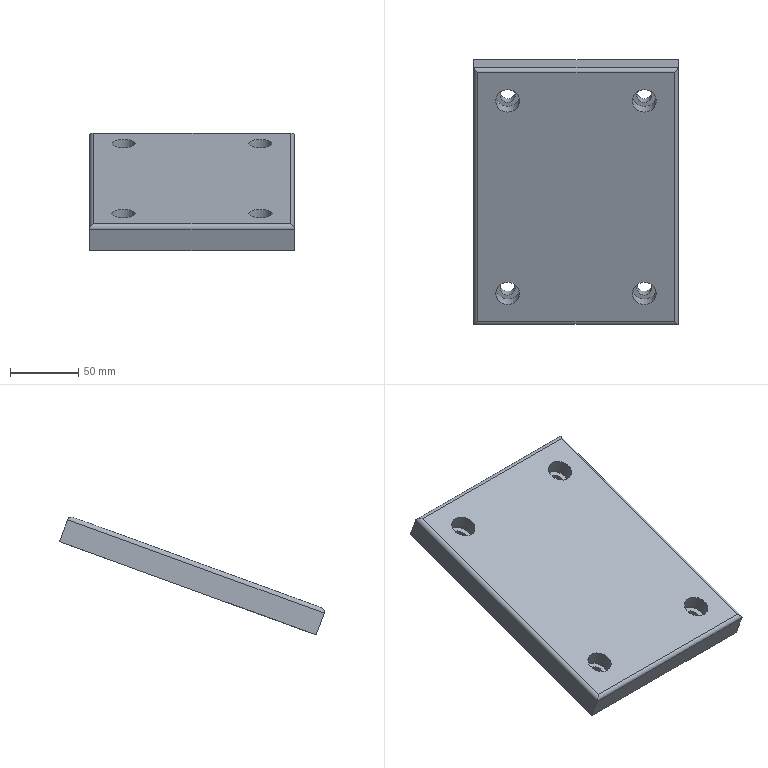Part | NX | features solid 2 | 1 solid | 22 faces | box 150 x 193.934 x 86.353 mm | volume 584072 mm3 | cylinder 12 | plane 10 | commonest cylinder face diameters 6 x4 11 x4 17.5 x4
STEP:
#1=CARTESIAN_POINT('',(72.,812.613,-309.301));
#2=VERTEX_POINT('',#1);
#3=CARTESIAN_POINT('',(-72.,812.613,-309.301));
#4=VERTEX_POINT('',#3);
#5=CARTESIAN_POINT('',(-37.6,812.613,-309.301));
#6=DIRECTION('',(-1.,0.,0.));
#7=VECTOR('',#6,1000.);
#8=LINE('',#5,#7);
#9=EDGE_CURVE('',#2,#4,#8,.T.);
#10=ORIENTED_EDGE('',*,*,#9,.T.);
#11=CARTESIAN_POINT('',(-75.,810.82,-313.146));
#12=VERTEX_POINT('',#11);
#13=CARTESIAN_POINT('',(-72.,813.639,-312.12));
#14=DIRECTION('',(0.7071,-0.6645,-0.2418));
#15=DIRECTION('',(-0.7071,-0.6645,-0.2418));
#16=AXIS2_PLACEMENT_3D('',#13,#14,#15);
#17=ELLIPSE('',#16,4.243,3.);
#18=EDGE_CURVE('',#4,#12,#17,.T.);
#19=ORIENTED_EDGE('',*,*,#18,.T.);
#20=CARTESIAN_POINT('',(75.,810.82,-313.146));
#21=VERTEX_POINT('',#20);
#22=CARTESIAN_POINT('',(78.95,810.82,-313.146));
#23=DIRECTION('',(-1.,0.,0.));
#24=VECTOR('',#23,1000.);
#25=LINE('',#22,#24);
#26=EDGE_CURVE('',#12,#21,#25,.F.);
#27=ORIENTED_EDGE('',*,*,#26,.T.);
#28=CARTESIAN_POINT('',(72.,813.639,-312.12));
#29=DIRECTION('',(0.7071,0.6645,0.2418));
#30=DIRECTION('',(0.7071,-0.6645,-0.2418));
#31=AXIS2_PLACEMENT_3D('',#28,#29,#30);
#32=ELLIPSE('',#31,4.243,3.);
#33=EDGE_CURVE('',#2,#21,#32,.T.);
#34=ORIENTED_EDGE('',*,*,#33,.F.);
#35=EDGE_LOOP('',(#10,#19,#27,#34));
#36=FACE_BOUND('',#35,.T.);
#37=CARTESIAN_POINT('',(-37.6,813.639,-312.12));
#38=DIRECTION('',(-1.,0.,0.));
#39=DIRECTION('',(0.,1.,0.));
#40=AXIS2_PLACEMENT_3D('',#37,#38,#39);
#41=CYLINDRICAL_SURFACE('',#40,3.);
#42=ADVANCED_FACE('',(#36),#41,.T.);
#43=CARTESIAN_POINT('',(-50.,966.018,-253.466));
#44=VERTEX_POINT('',#43);
#45=CARTESIAN_POINT('',(-50.,974.24,-250.474));
#46=DIRECTION('',(0.,0.342,-0.9397));
#47=DIRECTION('',(0.,-0.9397,-0.342));
#48=AXIS2_PLACEMENT_3D('',#45,#46,#47);
#49=CIRCLE('',#48,8.75);
#50=EDGE_CURVE('',#44,#44,#49,.F.);
#51=ORIENTED_EDGE('',*,*,#50,.F.);
#52=EDGE_LOOP('',(#51));
#53=FACE_BOUND('',#52,.T.);
#54=CARTESIAN_POINT('',(-50.,841.508,-298.784));
#55=VERTEX_POINT('',#54);
#56=CARTESIAN_POINT('',(-50.,833.286,-301.777));
#57=DIRECTION('',(0.,-0.342,0.9397));
#58=DIRECTION('',(0.,0.9397,0.342));
#59=AXIS2_PLACEMENT_3D('',#56,#57,#58);
#60=CIRCLE('',#59,8.75);
#61=EDGE_CURVE('',#55,#55,#60,.T.);
#62=ORIENTED_EDGE('',*,*,#61,.F.);
#63=EDGE_LOOP('',(#62));
#64=FACE_BOUND('',#63,.T.);
#65=CARTESIAN_POINT('',(-72.,994.913,-242.949));
#66=VERTEX_POINT('',#65);
#67=CARTESIAN_POINT('',(72.,994.913,-242.949));
#68=VERTEX_POINT('',#67);
#69=CARTESIAN_POINT('',(-37.6,994.913,-242.949));
#70=DIRECTION('',(-1.,0.,0.));
#71=VECTOR('',#70,1000.);
#72=LINE('',#69,#71);
#73=EDGE_CURVE('',#66,#68,#72,.F.);
#74=ORIENTED_EDGE('',*,*,#73,.F.);
#75=CARTESIAN_POINT('',(-72.,809.606,-310.396));
#76=DIRECTION('',(0.,0.9397,0.342));
#77=VECTOR('',#76,1000.);
#78=LINE('',#75,#77);
#79=EDGE_CURVE('',#4,#66,#78,.T.);
#80=ORIENTED_EDGE('',*,*,#79,.F.);
#81=ORIENTED_EDGE('',*,*,#9,.F.);
#82=CARTESIAN_POINT('',(72.,809.606,-310.396));
#83=DIRECTION('',(0.,0.9397,0.342));
#84=VECTOR('',#83,1000.);
#85=LINE('',#82,#84);
#86=EDGE_CURVE('',#2,#68,#85,.T.);
#87=ORIENTED_EDGE('',*,*,#86,.T.);
#88=EDGE_LOOP('',(#74,#80,#81,#87));
#89=FACE_BOUND('',#88,.T.);
#90=CARTESIAN_POINT('',(50.,966.018,-253.466));
#91=VERTEX_POINT('',#90);
#92=CARTESIAN_POINT('',(50.,974.24,-250.474));
#93=DIRECTION('',(0.,-0.342,0.9397));
#94=DIRECTION('',(0.,-0.9397,-0.342));
#95=AXIS2_PLACEMENT_3D('',#92,#93,#94);
#96=CIRCLE('',#95,8.75);
#97=EDGE_CURVE('',#91,#91,#96,.F.);
#98=ORIENTED_EDGE('',*,*,#97,.T.);
#99=EDGE_LOOP('',(#98));
#100=FACE_BOUND('',#99,.T.);
#101=CARTESIAN_POINT('',(50.,841.508,-298.784));
#102=VERTEX_POINT('',#101);
#103=CARTESIAN_POINT('',(50.,833.286,-301.777));
#104=DIRECTION('',(0.,0.342,-0.9397));
#105=DIRECTION('',(0.,0.9397,0.342));
#106=AXIS2_PLACEMENT_3D('',#103,#104,#105);
#107=CIRCLE('',#106,8.75);
#108=EDGE_CURVE('',#102,#102,#107,.T.);
#109=ORIENTED_EDGE('',*,*,#108,.T.);
#110=EDGE_LOOP('',(#109));
#111=FACE_BOUND('',#110,.T.);
#112=CARTESIAN_POINT('',(-37.6,809.606,-310.396));
#113=DIRECTION('',(0.,-0.342,0.9397));
#114=DIRECTION('',(0.,0.9397,0.342));
#115=AXIS2_PLACEMENT_3D('',#112,#113,#114);
#116=PLANE('',#115);
#117=ADVANCED_FACE('',(#53,#64,#89,#100,#111),#116,.T.);
#118=ORIENTED_EDGE('',*,*,#26,.F.);
#119=CARTESIAN_POINT('',(-75.,816.634,-329.121));
#120=VERTEX_POINT('',#119);
#121=CARTESIAN_POINT('',(-75.,817.01,-330.155));
#122=DIRECTION('',(0.,-0.342,0.9397));
#123=VECTOR('',#122,1000.);
#124=LINE('',#121,#123);
#125=EDGE_CURVE('',#120,#12,#124,.T.);
#126=ORIENTED_EDGE('',*,*,#125,.F.);
#127=CARTESIAN_POINT('',(75.,816.634,-329.121));
#128=VERTEX_POINT('',#127);
#129=CARTESIAN_POINT('',(-37.5,816.634,-329.121));
#130=DIRECTION('',(1.,0.,0.));
#131=VECTOR('',#130,1000.);
#132=LINE('',#129,#131);
#133=EDGE_CURVE('',#120,#128,#132,.T.);
#134=ORIENTED_EDGE('',*,*,#133,.T.);
#135=CARTESIAN_POINT('',(75.,817.01,-330.155));
#136=DIRECTION('',(0.,-0.342,0.9397));
#137=VECTOR('',#136,1000.);
#138=LINE('',#135,#137);
#139=EDGE_CURVE('',#128,#21,#138,.T.);
#140=ORIENTED_EDGE('',*,*,#139,.T.);
#141=EDGE_LOOP('',(#118,#126,#134,#140));
#142=FACE_BOUND('',#141,.T.);
#143=CARTESIAN_POINT('',(78.95,817.01,-330.155));
#144=DIRECTION('',(0.,-0.9397,-0.342));
#145=DIRECTION('',(-1.,0.,0.));
#146=AXIS2_PLACEMENT_3D('',#143,#144,#145);
#147=PLANE('',#146);
#148=ADVANCED_FACE('',(#142),#147,.T.);
#149=CARTESIAN_POINT('',(-50.,986.249,-267.387));
#150=VERTEX_POINT('',#149);
#151=CARTESIAN_POINT('',(-50.,981.08,-269.268));
#152=DIRECTION('',(0.,-0.342,0.9397));
#153=DIRECTION('',(0.,0.9397,0.342));
#154=AXIS2_PLACEMENT_3D('',#151,#152,#153);
#155=CIRCLE('',#154,5.5);
#156=EDGE_CURVE('',#150,#150,#155,.T.);
#157=ORIENTED_EDGE('',*,*,#156,.T.);
#158=EDGE_LOOP('',(#157));
#159=FACE_BOUND('',#158,.T.);
#160=CARTESIAN_POINT('',(-50.,845.295,-318.69));
#161=VERTEX_POINT('',#160);
#162=CARTESIAN_POINT('',(-50.,840.126,-320.571));
#163=DIRECTION('',(0.,-0.342,0.9397));
#164=DIRECTION('',(0.,0.9397,0.342));
#165=AXIS2_PLACEMENT_3D('',#162,#163,#164);
#166=CIRCLE('',#165,5.5);
#167=EDGE_CURVE('',#161,#161,#166,.T.);
#168=ORIENTED_EDGE('',*,*,#167,.T.);
#169=EDGE_LOOP('',(#168));
#170=FACE_BOUND('',#169,.T.);
#171=ORIENTED_EDGE('',*,*,#133,.F.);
#172=CARTESIAN_POINT('',(-75.,1004.573,-260.717));
#173=VERTEX_POINT('',#172);
#174=CARTESIAN_POINT('',(-75.,816.446,-329.19));
#175=DIRECTION('',(0.,-0.9397,-0.342));
#176=VECTOR('',#175,1000.);
#177=LINE('',#174,#176);
#178=EDGE_CURVE('',#173,#120,#177,.T.);
#179=ORIENTED_EDGE('',*,*,#178,.F.);
#180=CARTESIAN_POINT('',(75.,1004.573,-260.717));
#181=VERTEX_POINT('',#180);
#182=CARTESIAN_POINT('',(61.6,1004.573,-260.717));
#183=DIRECTION('',(1.,0.,0.));
#184=VECTOR('',#183,1000.);
#185=LINE('',#182,#184);
#186=EDGE_CURVE('',#173,#181,#185,.T.);
#187=ORIENTED_EDGE('',*,*,#186,.T.);
#188=CARTESIAN_POINT('',(75.,816.446,-329.19));
#189=DIRECTION('',(0.,-0.9397,-0.342));
#190=VECTOR('',#189,1000.);
#191=LINE('',#188,#190);
#192=EDGE_CURVE('',#181,#128,#191,.T.);
#193=ORIENTED_EDGE('',*,*,#192,.T.);
#194=EDGE_LOOP('',(#171,#179,#187,#193));
#195=FACE_BOUND('',#194,.T.);
#196=CARTESIAN_POINT('',(50.,986.249,-267.387));
#197=VERTEX_POINT('',#196);
#198=CARTESIAN_POINT('',(50.,981.08,-269.268));
#199=DIRECTION('',(0.,0.342,-0.9397));
#200=DIRECTION('',(0.,0.9397,0.342));
#201=AXIS2_PLACEMENT_3D('',#198,#199,#200);
#202=CIRCLE('',#201,5.5);
#203=EDGE_CURVE('',#197,#197,#202,.T.);
#204=ORIENTED_EDGE('',*,*,#203,.F.);
#205=EDGE_LOOP('',(#204));
#206=FACE_BOUND('',#205,.T.);
#207=CARTESIAN_POINT('',(50.,845.295,-318.69));
#208=VERTEX_POINT('',#207);
#209=CARTESIAN_POINT('',(50.,840.126,-320.571));
#210=DIRECTION('',(0.,0.342,-0.9397));
#211=DIRECTION('',(0.,0.9397,0.342));
#212=AXIS2_PLACEMENT_3D('',#209,#210,#211);
#213=CIRCLE('',#212,5.5);
#214=EDGE_CURVE('',#208,#208,#213,.T.);
#215=ORIENTED_EDGE('',*,*,#214,.F.);
#216=EDGE_LOOP('',(#215));
#217=FACE_BOUND('',#216,.T.);
#218=CARTESIAN_POINT('',(79.05,816.446,-329.19));
#219=DIRECTION('',(0.,0.342,-0.9397));
#220=DIRECTION('',(0.,0.9397,0.342));
#221=AXIS2_PLACEMENT_3D('',#218,#219,#220);
#222=PLANE('',#221);
#223=ADVANCED_FACE('',(#159,#170,#195,#206,#217),#222,.T.);
#224=ORIENTED_EDGE('',*,*,#186,.F.);
#225=CARTESIAN_POINT('',(-75.,998.758,-244.742));
#226=VERTEX_POINT('',#225);
#227=CARTESIAN_POINT('',(-75.,997.698,-241.829));
#228=DIRECTION('',(0.,0.342,-0.9397));
#229=VECTOR('',#228,1000.);
#230=LINE('',#227,#229);
#231=EDGE_CURVE('',#226,#173,#230,.T.);
#232=ORIENTED_EDGE('',*,*,#231,.F.);
#233=CARTESIAN_POINT('',(75.,998.758,-244.742));
#234=VERTEX_POINT('',#233);
#235=CARTESIAN_POINT('',(61.6,998.758,-244.742));
#236=DIRECTION('',(-1.,0.,0.));
#237=VECTOR('',#236,1000.);
#238=LINE('',#235,#237);
#239=EDGE_CURVE('',#234,#226,#238,.T.);
#240=ORIENTED_EDGE('',*,*,#239,.F.);
#241=CARTESIAN_POINT('',(75.,997.698,-241.829));
#242=DIRECTION('',(0.,0.342,-0.9397));
#243=VECTOR('',#242,1000.);
#244=LINE('',#241,#243);
#245=EDGE_CURVE('',#234,#181,#244,.T.);
#246=ORIENTED_EDGE('',*,*,#245,.T.);
#247=EDGE_LOOP('',(#224,#232,#240,#246));
#248=FACE_BOUND('',#247,.T.);
#249=CARTESIAN_POINT('',(61.6,997.698,-241.829));
#250=DIRECTION('',(0.,0.9397,0.342));
#251=DIRECTION('',(-1.,0.,0.));
#252=AXIS2_PLACEMENT_3D('',#249,#250,#251);
#253=PLANE('',#252);
#254=ADVANCED_FACE('',(#248),#253,.T.);
#255=ORIENTED_EDGE('',*,*,#239,.T.);
#256=CARTESIAN_POINT('',(-72.,995.939,-245.768));
#257=DIRECTION('',(-0.7071,-0.6645,-0.2418));
#258=DIRECTION('',(-0.7071,0.6645,0.2418));
#259=AXIS2_PLACEMENT_3D('',#256,#257,#258);
#260=ELLIPSE('',#259,4.243,3.);
#261=EDGE_CURVE('',#66,#226,#260,.T.);
#262=ORIENTED_EDGE('',*,*,#261,.F.);
#263=ORIENTED_EDGE('',*,*,#73,.T.);
#264=CARTESIAN_POINT('',(72.,995.939,-245.768));
#265=DIRECTION('',(-0.7071,0.6645,0.2418));
#266=DIRECTION('',(0.7071,0.6645,0.2418));
#267=AXIS2_PLACEMENT_3D('',#264,#265,#266);
#268=ELLIPSE('',#267,4.243,3.);
#269=EDGE_CURVE('',#68,#234,#268,.T.);
#270=ORIENTED_EDGE('',*,*,#269,.T.);
#271=EDGE_LOOP('',(#255,#262,#263,#270));
#272=FACE_BOUND('',#271,.T.);
#273=CARTESIAN_POINT('',(61.6,995.939,-245.768));
#274=DIRECTION('',(-1.,0.,0.));
#275=DIRECTION('',(0.,1.,0.));
#276=AXIS2_PLACEMENT_3D('',#273,#274,#275);
#277=CYLINDRICAL_SURFACE('',#276,3.);
#278=ADVANCED_FACE('',(#272),#277,.T.);
#279=ORIENTED_EDGE('',*,*,#231,.T.);
#280=ORIENTED_EDGE('',*,*,#178,.T.);
#281=ORIENTED_EDGE('',*,*,#125,.T.);
#282=CARTESIAN_POINT('',(-75.,803.772,-315.712));
#283=DIRECTION('',(0.,0.9397,0.342));
#284=VECTOR('',#283,1000.);
#285=LINE('',#282,#284);
#286=EDGE_CURVE('',#226,#12,#285,.F.);
#287=ORIENTED_EDGE('',*,*,#286,.F.);
#288=EDGE_LOOP('',(#279,#280,#281,#287));
#289=FACE_BOUND('',#288,.T.);
#290=CARTESIAN_POINT('',(-75.,809.928,-332.626));
#291=DIRECTION('',(-1.,0.,0.));
#292=DIRECTION('',(0.,0.9397,0.342));
#293=AXIS2_PLACEMENT_3D('',#290,#291,#292);
#294=PLANE('',#293);
#295=ADVANCED_FACE('',(#289),#294,.T.);
#296=ORIENTED_EDGE('',*,*,#167,.F.);
#297=EDGE_LOOP('',(#296));
#298=FACE_BOUND('',#297,.T.);
#299=CARTESIAN_POINT('',(-50.,842.558,-311.172));
#300=VERTEX_POINT('',#299);
#301=CARTESIAN_POINT('',(-50.,837.39,-313.053));
#302=DIRECTION('',(0.,-0.342,0.9397));
#303=DIRECTION('',(0.,0.9397,0.342));
#304=AXIS2_PLACEMENT_3D('',#301,#302,#303);
#305=CIRCLE('',#304,5.5);
#306=EDGE_CURVE('',#300,#300,#305,.T.);
#307=ORIENTED_EDGE('',*,*,#306,.T.);
#308=EDGE_LOOP('',(#307));
#309=FACE_BOUND('',#308,.T.);
#310=CARTESIAN_POINT('',(-50.,850.387,-348.761));
#311=DIRECTION('',(0.,0.342,-0.9397));
#312=DIRECTION('',(0.,0.9397,0.342));
#313=AXIS2_PLACEMENT_3D('',#310,#311,#312);
#314=CYLINDRICAL_SURFACE('',#313,5.5);
#315=ADVANCED_FACE('',(#298,#309),#314,.F.);
#316=ORIENTED_EDGE('',*,*,#306,.F.);
#317=EDGE_LOOP('',(#316));
#318=FACE_BOUND('',#317,.T.);
#319=CARTESIAN_POINT('',(-50.,845.612,-310.06));
#320=VERTEX_POINT('',#319);
#321=CARTESIAN_POINT('',(-50.,837.39,-313.053));
#322=DIRECTION('',(0.,-0.342,0.9397));
#323=DIRECTION('',(0.,0.9397,0.342));
#324=AXIS2_PLACEMENT_3D('',#321,#322,#323);
#325=CIRCLE('',#324,8.75);
#326=EDGE_CURVE('',#320,#320,#325,.T.);
#327=ORIENTED_EDGE('',*,*,#326,.T.);
#328=EDGE_LOOP('',(#327));
#329=FACE_BOUND('',#328,.T.);
#330=CARTESIAN_POINT('',(-38.,837.39,-313.053));
#331=DIRECTION('',(0.,0.342,-0.9397));
#332=DIRECTION('',(0.,0.9397,0.342));
#333=AXIS2_PLACEMENT_3D('',#330,#331,#332);
#334=PLANE('',#333);
#335=ADVANCED_FACE('',(#318,#329),#334,.F.);
#336=ORIENTED_EDGE('',*,*,#326,.F.);
#337=EDGE_LOOP('',(#336));
#338=FACE_BOUND('',#337,.T.);
#339=ORIENTED_EDGE('',*,*,#61,.T.);
#340=EDGE_LOOP('',(#339));
#341=FACE_BOUND('',#340,.T.);
#342=CARTESIAN_POINT('',(-50.,833.286,-301.777));
#343=DIRECTION('',(0.,0.342,-0.9397));
#344=DIRECTION('',(0.,0.9397,0.342));
#345=AXIS2_PLACEMENT_3D('',#342,#343,#344);
#346=CYLINDRICAL_SURFACE('',#345,8.75);
#347=ADVANCED_FACE('',(#338,#341),#346,.F.);
#348=ORIENTED_EDGE('',*,*,#156,.F.);
#349=EDGE_LOOP('',(#348));
#350=FACE_BOUND('',#349,.T.);
#351=CARTESIAN_POINT('',(-50.,983.512,-259.869));
#352=VERTEX_POINT('',#351);
#353=CARTESIAN_POINT('',(-50.,978.344,-261.75));
#354=DIRECTION('',(0.,-0.342,0.9397));
#355=DIRECTION('',(0.,0.9397,0.342));
#356=AXIS2_PLACEMENT_3D('',#353,#354,#355);
#357=CIRCLE('',#356,5.5);
#358=EDGE_CURVE('',#352,#352,#357,.T.);
#359=ORIENTED_EDGE('',*,*,#358,.T.);
#360=EDGE_LOOP('',(#359));
#361=FACE_BOUND('',#360,.T.);
#362=CARTESIAN_POINT('',(-50.,991.341,-297.458));
#363=DIRECTION('',(0.,0.342,-0.9397));
#364=DIRECTION('',(0.,0.9397,0.342));
#365=AXIS2_PLACEMENT_3D('',#362,#363,#364);
#366=CYLINDRICAL_SURFACE('',#365,5.5);
#367=ADVANCED_FACE('',(#350,#361),#366,.F.);
#368=ORIENTED_EDGE('',*,*,#358,.F.);
#369=EDGE_LOOP('',(#368));
#370=FACE_BOUND('',#369,.T.);
#371=CARTESIAN_POINT('',(-50.,986.566,-258.757));
#372=VERTEX_POINT('',#371);
#373=CARTESIAN_POINT('',(-50.,978.344,-261.75));
#374=DIRECTION('',(0.,-0.342,0.9397));
#375=DIRECTION('',(0.,0.9397,0.342));
#376=AXIS2_PLACEMENT_3D('',#373,#374,#375);
#377=CIRCLE('',#376,8.75);
#378=EDGE_CURVE('',#372,#372,#377,.T.);
#379=ORIENTED_EDGE('',*,*,#378,.T.);
#380=EDGE_LOOP('',(#379));
#381=FACE_BOUND('',#380,.T.);
#382=CARTESIAN_POINT('',(-38.,978.344,-261.75));
#383=DIRECTION('',(0.,0.342,-0.9397));
#384=DIRECTION('',(0.,0.9397,0.342));
#385=AXIS2_PLACEMENT_3D('',#382,#383,#384);
#386=PLANE('',#385);
#387=ADVANCED_FACE('',(#370,#381),#386,.F.);
#388=ORIENTED_EDGE('',*,*,#378,.F.);
#389=EDGE_LOOP('',(#388));
#390=FACE_BOUND('',#389,.T.);
#391=ORIENTED_EDGE('',*,*,#50,.T.);
#392=EDGE_LOOP('',(#391));
#393=FACE_BOUND('',#392,.T.);
#394=CARTESIAN_POINT('',(-50.,974.24,-250.474));
#395=DIRECTION('',(0.,0.342,-0.9397));
#396=DIRECTION('',(0.,0.9397,0.342));
#397=AXIS2_PLACEMENT_3D('',#394,#395,#396);
#398=CYLINDRICAL_SURFACE('',#397,8.75);
#399=ADVANCED_FACE('',(#390,#393),#398,.F.);
#400=ORIENTED_EDGE('',*,*,#18,.F.);
#401=ORIENTED_EDGE('',*,*,#79,.T.);
#402=ORIENTED_EDGE('',*,*,#261,.T.);
#403=ORIENTED_EDGE('',*,*,#286,.T.);
#404=EDGE_LOOP('',(#400,#401,#402,#403));
#405=FACE_BOUND('',#404,.T.);
#406=CARTESIAN_POINT('',(-72.,810.632,-313.215));
#407=DIRECTION('',(0.,0.9397,0.342));
#408=DIRECTION('',(0.,-0.342,0.9397));
#409=AXIS2_PLACEMENT_3D('',#406,#407,#408);
#410=CYLINDRICAL_SURFACE('',#409,3.);
#411=ADVANCED_FACE('',(#405),#410,.T.);
#412=ORIENTED_EDGE('',*,*,#245,.F.);
#413=CARTESIAN_POINT('',(75.,803.772,-315.712));
#414=DIRECTION('',(0.,0.9397,0.342));
#415=VECTOR('',#414,1000.);
#416=LINE('',#413,#415);
#417=EDGE_CURVE('',#234,#21,#416,.F.);
#418=ORIENTED_EDGE('',*,*,#417,.T.);
#419=ORIENTED_EDGE('',*,*,#139,.F.);
#420=ORIENTED_EDGE('',*,*,#192,.F.);
#421=EDGE_LOOP('',(#412,#418,#419,#420));
#422=FACE_BOUND('',#421,.T.);
#423=CARTESIAN_POINT('',(75.,809.928,-332.626));
#424=DIRECTION('',(1.,0.,0.));
#425=DIRECTION('',(0.,0.9397,0.342));
#426=AXIS2_PLACEMENT_3D('',#423,#424,#425);
#427=PLANE('',#426);
#428=ADVANCED_FACE('',(#422),#427,.T.);
#429=ORIENTED_EDGE('',*,*,#214,.T.);
#430=EDGE_LOOP('',(#429));
#431=FACE_BOUND('',#430,.T.);
#432=CARTESIAN_POINT('',(50.,842.558,-311.172));
#433=VERTEX_POINT('',#432);
#434=CARTESIAN_POINT('',(50.,837.39,-313.053));
#435=DIRECTION('',(0.,0.342,-0.9397));
#436=DIRECTION('',(0.,0.9397,0.342));
#437=AXIS2_PLACEMENT_3D('',#434,#435,#436);
#438=CIRCLE('',#437,5.5);
#439=EDGE_CURVE('',#433,#433,#438,.T.);
#440=ORIENTED_EDGE('',*,*,#439,.F.);
#441=EDGE_LOOP('',(#440));
#442=FACE_BOUND('',#441,.T.);
#443=CARTESIAN_POINT('',(50.,850.387,-348.761));
#444=DIRECTION('',(0.,0.342,-0.9397));
#445=DIRECTION('',(0.,0.9397,0.342));
#446=AXIS2_PLACEMENT_3D('',#443,#444,#445);
#447=CYLINDRICAL_SURFACE('',#446,5.5);
#448=ADVANCED_FACE('',(#431,#442),#447,.F.);
#449=ORIENTED_EDGE('',*,*,#439,.T.);
#450=EDGE_LOOP('',(#449));
#451=FACE_BOUND('',#450,.T.);
#452=CARTESIAN_POINT('',(50.,845.612,-310.06));
#453=VERTEX_POINT('',#452);
#454=CARTESIAN_POINT('',(50.,837.39,-313.053));
#455=DIRECTION('',(0.,0.342,-0.9397));
#456=DIRECTION('',(0.,0.9397,0.342));
#457=AXIS2_PLACEMENT_3D('',#454,#455,#456);
#458=CIRCLE('',#457,8.75);
#459=EDGE_CURVE('',#453,#453,#458,.T.);
#460=ORIENTED_EDGE('',*,*,#459,.F.);
#461=EDGE_LOOP('',(#460));
#462=FACE_BOUND('',#461,.T.);
#463=CARTESIAN_POINT('',(63.,837.39,-313.053));
#464=DIRECTION('',(0.,0.342,-0.9397));
#465=DIRECTION('',(0.,0.9397,0.342));
#466=AXIS2_PLACEMENT_3D('',#463,#464,#465);
#467=PLANE('',#466);
#468=ADVANCED_FACE('',(#451,#462),#467,.F.);
#469=ORIENTED_EDGE('',*,*,#459,.T.);
#470=EDGE_LOOP('',(#469));
#471=FACE_BOUND('',#470,.T.);
#472=ORIENTED_EDGE('',*,*,#108,.F.);
#473=EDGE_LOOP('',(#472));
#474=FACE_BOUND('',#473,.T.);
#475=CARTESIAN_POINT('',(50.,833.286,-301.777));
#476=DIRECTION('',(0.,0.342,-0.9397));
#477=DIRECTION('',(0.,0.9397,0.342));
#478=AXIS2_PLACEMENT_3D('',#475,#476,#477);
#479=CYLINDRICAL_SURFACE('',#478,8.75);
#480=ADVANCED_FACE('',(#471,#474),#479,.F.);
#481=ORIENTED_EDGE('',*,*,#203,.T.);
#482=EDGE_LOOP('',(#481));
#483=FACE_BOUND('',#482,.T.);
#484=CARTESIAN_POINT('',(50.,983.512,-259.869));
#485=VERTEX_POINT('',#484);
#486=CARTESIAN_POINT('',(50.,978.344,-261.75));
#487=DIRECTION('',(0.,0.342,-0.9397));
#488=DIRECTION('',(0.,0.9397,0.342));
#489=AXIS2_PLACEMENT_3D('',#486,#487,#488);
#490=CIRCLE('',#489,5.5);
#491=EDGE_CURVE('',#485,#485,#490,.T.);
#492=ORIENTED_EDGE('',*,*,#491,.F.);
#493=EDGE_LOOP('',(#492));
#494=FACE_BOUND('',#493,.T.);
#495=CARTESIAN_POINT('',(50.,991.341,-297.458));
#496=DIRECTION('',(0.,0.342,-0.9397));
#497=DIRECTION('',(0.,0.9397,0.342));
#498=AXIS2_PLACEMENT_3D('',#495,#496,#497);
#499=CYLINDRICAL_SURFACE('',#498,5.5);
#500=ADVANCED_FACE('',(#483,#494),#499,.F.);
#501=ORIENTED_EDGE('',*,*,#491,.T.);
#502=EDGE_LOOP('',(#501));
#503=FACE_BOUND('',#502,.T.);
#504=CARTESIAN_POINT('',(50.,986.566,-258.757));
#505=VERTEX_POINT('',#504);
#506=CARTESIAN_POINT('',(50.,978.344,-261.75));
#507=DIRECTION('',(0.,0.342,-0.9397));
#508=DIRECTION('',(0.,0.9397,0.342));
#509=AXIS2_PLACEMENT_3D('',#506,#507,#508);
#510=CIRCLE('',#509,8.75);
#511=EDGE_CURVE('',#505,#505,#510,.T.);
#512=ORIENTED_EDGE('',*,*,#511,.F.);
#513=EDGE_LOOP('',(#512));
#514=FACE_BOUND('',#513,.T.);
#515=CARTESIAN_POINT('',(63.,978.344,-261.75));
#516=DIRECTION('',(0.,0.342,-0.9397));
#517=DIRECTION('',(0.,0.9397,0.342));
#518=AXIS2_PLACEMENT_3D('',#515,#516,#517);
#519=PLANE('',#518);
#520=ADVANCED_FACE('',(#503,#514),#519,.F.);
#521=ORIENTED_EDGE('',*,*,#511,.T.);
#522=EDGE_LOOP('',(#521));
#523=FACE_BOUND('',#522,.T.);
#524=ORIENTED_EDGE('',*,*,#97,.F.);
#525=EDGE_LOOP('',(#524));
#526=FACE_BOUND('',#525,.T.);
#527=CARTESIAN_POINT('',(50.,974.24,-250.474));
#528=DIRECTION('',(0.,0.342,-0.9397));
#529=DIRECTION('',(0.,0.9397,0.342));
#530=AXIS2_PLACEMENT_3D('',#527,#528,#529);
#531=CYLINDRICAL_SURFACE('',#530,8.75);
#532=ADVANCED_FACE('',(#523,#526),#531,.F.);
#533=ORIENTED_EDGE('',*,*,#33,.T.);
#534=ORIENTED_EDGE('',*,*,#417,.F.);
#535=ORIENTED_EDGE('',*,*,#269,.F.);
#536=ORIENTED_EDGE('',*,*,#86,.F.);
#537=EDGE_LOOP('',(#533,#534,#535,#536));
#538=FACE_BOUND('',#537,.T.);
#539=CARTESIAN_POINT('',(72.,810.632,-313.215));
#540=DIRECTION('',(0.,0.9397,0.342));
#541=DIRECTION('',(0.,-0.342,0.9397));
#542=AXIS2_PLACEMENT_3D('',#539,#540,#541);
#543=CYLINDRICAL_SURFACE('',#542,3.);
#544=ADVANCED_FACE('',(#538),#543,.T.);
#545=CLOSED_SHELL('',(#42,#117,#148,#223,#254,#278,#295,#315,#335,#347,#367,#387,#399,#411,#428,#448,#468,#480,#500,#520,#532,#544));
#546=MANIFOLD_SOLID_BREP('',#545);
#547=(LENGTH_UNIT()NAMED_UNIT(*)SI_UNIT(.MILLI.,.METRE.));
#548=UNCERTAINTY_MEASURE_WITH_UNIT(LENGTH_MEASURE(0.00001),#547,'','');
#549=(NAMED_UNIT(*)PLANE_ANGLE_UNIT()SI_UNIT($,.RADIAN.));
#550=(NAMED_UNIT(*)SI_UNIT($,.STERADIAN.)SOLID_ANGLE_UNIT());
#551=(GEOMETRIC_REPRESENTATION_CONTEXT(3)GLOBAL_UNCERTAINTY_ASSIGNED_CONTEXT((#548))GLOBAL_UNIT_ASSIGNED_CONTEXT((#547,#549,#550))REPRESENTATION_CONTEXT('',''));
#552=ADVANCED_BREP_SHAPE_REPRESENTATION('',(#546),#551);